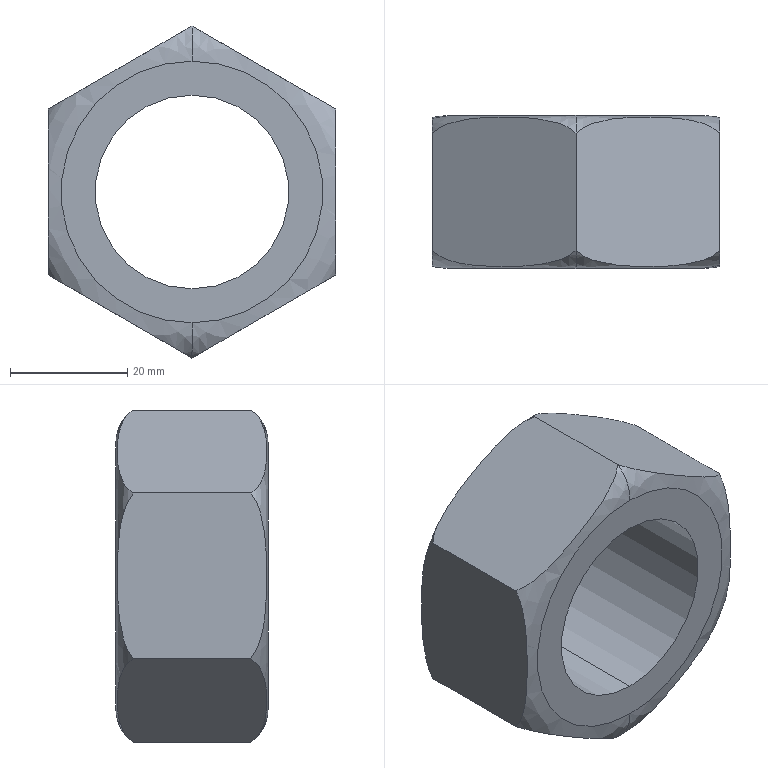Part | SolidWorks | features Extrusion 1, RevCut 1 | 1 solid | 14 faces | box 49 x 26 x 56.58 mm | volume 31477 mm3 | plane 8 | spline 4 | cylinder 2 | commonest cylinder face diameters 33 x2
STEP:
#1=CARTESIAN_POINT('',(0.,10.,-28.29));
#2=VERTEX_POINT('',#1);
#3=CARTESIAN_POINT('',(24.5,10.,-14.145));
#4=VERTEX_POINT('',#3);
#5=CARTESIAN_POINT('',(0.,10.,-28.29));
#6=CARTESIAN_POINT('',(0.412,10.401,-28.052));
#7=CARTESIAN_POINT('',(0.863,10.721,-27.792));
#8=CARTESIAN_POINT('',(1.576,11.123,-27.38));
#9=CARTESIAN_POINT('',(1.819,11.244,-27.24));
#10=CARTESIAN_POINT('',(2.317,11.465,-26.952));
#11=CARTESIAN_POINT('',(2.571,11.564,-26.806));
#12=CARTESIAN_POINT('',(3.333,11.832,-26.366));
#13=CARTESIAN_POINT('',(3.846,11.972,-26.069));
#14=CARTESIAN_POINT('',(4.88,12.204,-25.473));
#15=CARTESIAN_POINT('',(5.4,12.295,-25.173));
#16=CARTESIAN_POINT('',(6.967,12.519,-24.268));
#17=CARTESIAN_POINT('',(8.022,12.604,-23.659));
#18=CARTESIAN_POINT('',(10.136,12.711,-22.438));
#19=CARTESIAN_POINT('',(11.193,12.733,-21.828));
#20=CARTESIAN_POINT('',(13.306,12.733,-20.608));
#21=CARTESIAN_POINT('',(14.363,12.711,-19.998));
#22=CARTESIAN_POINT('',(16.475,12.604,-18.778));
#23=CARTESIAN_POINT('',(17.532,12.519,-18.168));
#24=CARTESIAN_POINT('',(19.105,12.294,-17.26));
#25=CARTESIAN_POINT('',(19.627,12.202,-16.958));
#26=CARTESIAN_POINT('',(20.667,11.969,-16.358));
#27=CARTESIAN_POINT('',(21.183,11.827,-16.06));
#28=CARTESIAN_POINT('',(22.191,11.472,-15.478));
#29=CARTESIAN_POINT('',(22.684,11.259,-15.193));
#30=CARTESIAN_POINT('',(23.399,10.855,-14.781));
#31=CARTESIAN_POINT('',(23.633,10.706,-14.646));
#32=CARTESIAN_POINT('',(24.081,10.378,-14.387));
#33=CARTESIAN_POINT('',(24.296,10.199,-14.263));
#34=CARTESIAN_POINT('',(24.5,10.,-14.145));
#35=B_SPLINE_CURVE_WITH_KNOTS('',3,(#5,#6,#7,#8,#9,#10,#11,#12,#13,#14,#15,#16,#17,#18,#19,#20,#21,#22,#23,#24,#25,#26,#27,#28,#29,#30,#31,#32,#33,#34),.UNSPECIFIED.,.F.,.F.,(4,2,2,2,2,2,2,2,2,2,2,2,2,2,4),(0.,0.00183,0.002745,0.003661,0.005491,0.007321,0.01098,0.01464,0.0183,0.02196,0.02379,0.02562,0.02745,0.02837,0.02929),.UNSPECIFIED.);
#36=EDGE_CURVE('',#2,#4,#35,.T.);
#37=ORIENTED_EDGE('',*,*,#36,.F.);
#38=CARTESIAN_POINT('',(0.,13.,-22.29));
#39=VERTEX_POINT('',#38);
#40=CARTESIAN_POINT('',(0.,10.,-28.29));
#41=CARTESIAN_POINT('',(0.,12.129,-27.029));
#42=CARTESIAN_POINT('',(0.,13.,-24.712));
#43=CARTESIAN_POINT('',(0.,13.,-22.29));
#44=B_SPLINE_CURVE_WITH_KNOTS('',3,(#40,#41,#42,#43),.UNSPECIFIED.,.F.,.F.,(4,4),(0.,1.),.UNSPECIFIED.);
#45=EDGE_CURVE('',#2,#39,#44,.T.);
#46=ORIENTED_EDGE('',*,*,#45,.T.);
#47=CARTESIAN_POINT('',(0.,13.,22.29));
#48=VERTEX_POINT('',#47);
#49=CARTESIAN_POINT('',(0.,13.,0.));
#50=DIRECTION('',(0.,1.,0.));
#51=DIRECTION('',(0.,0.,1.));
#52=AXIS2_PLACEMENT_3D('',#49,#50,#51);
#53=CIRCLE('',#52,22.29);
#54=EDGE_CURVE('',#48,#39,#53,.T.);
#55=ORIENTED_EDGE('',*,*,#54,.F.);
#56=CARTESIAN_POINT('',(0.,10.,28.29));
#57=VERTEX_POINT('',#56);
#58=CARTESIAN_POINT('',(0.,10.,28.29));
#59=CARTESIAN_POINT('',(0.,12.129,27.029));
#60=CARTESIAN_POINT('',(0.,13.,24.712));
#61=CARTESIAN_POINT('',(0.,13.,22.29));
#62=B_SPLINE_CURVE_WITH_KNOTS('',3,(#58,#59,#60,#61),.UNSPECIFIED.,.F.,.F.,(4,4),(0.,1.),.UNSPECIFIED.);
#63=EDGE_CURVE('',#57,#48,#62,.T.);
#64=ORIENTED_EDGE('',*,*,#63,.F.);
#65=CARTESIAN_POINT('',(24.5,10.,14.145));
#66=VERTEX_POINT('',#65);
#67=CARTESIAN_POINT('',(24.5,10.,14.145));
#68=CARTESIAN_POINT('',(24.088,10.401,14.383));
#69=CARTESIAN_POINT('',(23.637,10.721,14.643));
#70=CARTESIAN_POINT('',(22.924,11.123,15.055));
#71=CARTESIAN_POINT('',(22.681,11.244,15.196));
#72=CARTESIAN_POINT('',(22.183,11.465,15.483));
#73=CARTESIAN_POINT('',(21.929,11.564,15.629));
#74=CARTESIAN_POINT('',(21.167,11.832,16.069));
#75=CARTESIAN_POINT('',(20.654,11.972,16.366));
#76=CARTESIAN_POINT('',(19.62,12.204,16.962));
#77=CARTESIAN_POINT('',(19.1,12.295,17.263));
#78=CARTESIAN_POINT('',(17.533,12.519,18.168));
#79=CARTESIAN_POINT('',(16.478,12.604,18.777));
#80=CARTESIAN_POINT('',(14.364,12.711,19.997));
#81=CARTESIAN_POINT('',(13.307,12.733,20.607));
#82=CARTESIAN_POINT('',(11.194,12.733,21.827));
#83=CARTESIAN_POINT('',(10.137,12.711,22.437));
#84=CARTESIAN_POINT('',(8.025,12.604,23.657));
#85=CARTESIAN_POINT('',(6.968,12.519,24.267));
#86=CARTESIAN_POINT('',(5.395,12.294,25.175));
#87=CARTESIAN_POINT('',(4.873,12.202,25.477));
#88=CARTESIAN_POINT('',(3.833,11.969,26.077));
#89=CARTESIAN_POINT('',(3.317,11.827,26.375));
#90=CARTESIAN_POINT('',(2.309,11.472,26.957));
#91=CARTESIAN_POINT('',(1.816,11.259,27.242));
#92=CARTESIAN_POINT('',(1.101,10.855,27.654));
#93=CARTESIAN_POINT('',(0.867,10.706,27.79));
#94=CARTESIAN_POINT('',(0.419,10.378,28.048));
#95=CARTESIAN_POINT('',(0.2039,10.199,28.172));
#96=CARTESIAN_POINT('',(0.,10.,28.29));
#97=B_SPLINE_CURVE_WITH_KNOTS('',3,(#67,#68,#69,#70,#71,#72,#73,#74,#75,#76,#77,#78,#79,#80,#81,#82,#83,#84,#85,#86,#87,#88,#89,#90,#91,#92,#93,#94,#95,#96),.UNSPECIFIED.,.F.,.F.,(4,2,2,2,2,2,2,2,2,2,2,2,2,2,4),(0.,0.00183,0.002745,0.003661,0.005491,0.007321,0.01098,0.01464,0.0183,0.02196,0.02379,0.02562,0.02745,0.02837,0.02929),.UNSPECIFIED.);
#98=EDGE_CURVE('',#66,#57,#97,.T.);
#99=ORIENTED_EDGE('',*,*,#98,.F.);
#100=CARTESIAN_POINT('',(24.5,10.,-14.145));
#101=CARTESIAN_POINT('',(24.5,10.401,-13.669));
#102=CARTESIAN_POINT('',(24.5,10.721,-13.149));
#103=CARTESIAN_POINT('',(24.5,11.123,-12.326));
#104=CARTESIAN_POINT('',(24.5,11.244,-12.044));
#105=CARTESIAN_POINT('',(24.5,11.465,-11.469));
#106=CARTESIAN_POINT('',(24.5,11.564,-11.176));
#107=CARTESIAN_POINT('',(24.5,11.832,-10.296));
#108=CARTESIAN_POINT('',(24.5,11.972,-9.704));
#109=CARTESIAN_POINT('',(24.5,12.204,-8.51));
#110=CARTESIAN_POINT('',(24.5,12.295,-7.91));
#111=CARTESIAN_POINT('',(24.5,12.519,-6.1));
#112=CARTESIAN_POINT('',(24.5,12.604,-4.882));
#113=CARTESIAN_POINT('',(24.5,12.711,-2.441));
#114=CARTESIAN_POINT('',(24.5,12.733,-1.221));
#115=CARTESIAN_POINT('',(24.5,12.733,1.219));
#116=CARTESIAN_POINT('',(24.5,12.711,2.439));
#117=CARTESIAN_POINT('',(24.5,12.604,4.879));
#118=CARTESIAN_POINT('',(24.5,12.519,6.1));
#119=CARTESIAN_POINT('',(24.5,12.294,7.916));
#120=CARTESIAN_POINT('',(24.5,12.202,8.519));
#121=CARTESIAN_POINT('',(24.5,11.969,9.719));
#122=CARTESIAN_POINT('',(24.5,11.827,10.315));
#123=CARTESIAN_POINT('',(24.5,11.472,11.479));
#124=CARTESIAN_POINT('',(24.5,11.259,12.048));
#125=CARTESIAN_POINT('',(24.5,10.855,12.874));
#126=CARTESIAN_POINT('',(24.5,10.706,13.144));
#127=CARTESIAN_POINT('',(24.5,10.378,13.661));
#128=CARTESIAN_POINT('',(24.5,10.199,13.91));
#129=CARTESIAN_POINT('',(24.5,10.,14.145));
#130=B_SPLINE_CURVE_WITH_KNOTS('',3,(#100,#101,#102,#103,#104,#105,#106,#107,#108,#109,#110,#111,#112,#113,#114,#115,#116,#117,#118,#119,#120,#121,#122,#123,#124,#125,#126,#127,#128,#129),.UNSPECIFIED.,.F.,.F.,(4,2,2,2,2,2,2,2,2,2,2,2,2,2,4),(0.,0.00183,0.002745,0.003661,0.005491,0.007321,0.01098,0.01464,0.0183,0.02196,0.02379,0.02562,0.02745,0.02837,0.02929),.UNSPECIFIED.);
#131=EDGE_CURVE('',#4,#66,#130,.T.);
#132=ORIENTED_EDGE('',*,*,#131,.F.);
#133=EDGE_LOOP('',(#37,#46,#55,#64,#99,#132));
#134=FACE_OUTER_BOUND('',#133,.T.);
#135=CARTESIAN_POINT('',(0.,10.,28.29));
#136=CARTESIAN_POINT('',(56.58,10.,28.29));
#137=CARTESIAN_POINT('',(56.58,10.,-28.29));
#138=CARTESIAN_POINT('',(0.,10.,-28.29));
#139=CARTESIAN_POINT('',(0.,12.129,27.029));
#140=CARTESIAN_POINT('',(54.057,12.129,27.029));
#141=CARTESIAN_POINT('',(54.057,12.129,-27.029));
#142=CARTESIAN_POINT('',(0.,12.129,-27.029));
#143=CARTESIAN_POINT('',(0.,13.,24.712));
#144=CARTESIAN_POINT('',(49.423,13.,24.712));
#145=CARTESIAN_POINT('',(49.423,13.,-24.712));
#146=CARTESIAN_POINT('',(0.,13.,-24.712));
#147=CARTESIAN_POINT('',(0.,13.,22.29));
#148=CARTESIAN_POINT('',(44.58,13.,22.29));
#149=CARTESIAN_POINT('',(44.58,13.,-22.29));
#150=CARTESIAN_POINT('',(0.,13.,-22.29));
#151=(BOUNDED_SURFACE()B_SPLINE_SURFACE(3,3,((#135,#136,#137,#138),(#139,#140,#141,#142),(#143,#144,#145,#146),(#147,#148,#149,#150)),.UNSPECIFIED.,.F.,.F.,.F.)B_SPLINE_SURFACE_WITH_KNOTS((4,4),(4,4),(0.,1.),(0.,1.),.UNSPECIFIED.)GEOMETRIC_REPRESENTATION_ITEM()RATIONAL_B_SPLINE_SURFACE(((1.,0.3333,0.3333,1.),(1.,0.3333,0.3333,1.),(1.,0.3333,0.3333,1.),(1.,0.3333,0.3333,1.)))REPRESENTATION_ITEM('')SURFACE());
#152=ADVANCED_FACE('',(#134),#151,.F.);
#153=CARTESIAN_POINT('',(0.,-13.,22.29));
#154=VERTEX_POINT('',#153);
#155=CARTESIAN_POINT('',(0.,-13.,-22.29));
#156=VERTEX_POINT('',#155);
#157=CARTESIAN_POINT('',(0.,-13.,0.));
#158=DIRECTION('',(0.,1.,0.));
#159=DIRECTION('',(0.,0.,1.));
#160=AXIS2_PLACEMENT_3D('',#157,#158,#159);
#161=CIRCLE('',#160,22.29);
#162=EDGE_CURVE('',#154,#156,#161,.T.);
#163=ORIENTED_EDGE('',*,*,#162,.T.);
#164=CARTESIAN_POINT('',(0.,-10.,-28.29));
#165=VERTEX_POINT('',#164);
#166=CARTESIAN_POINT('',(0.,-13.,-22.29));
#167=CARTESIAN_POINT('',(0.,-13.,-24.712));
#168=CARTESIAN_POINT('',(0.,-12.129,-27.029));
#169=CARTESIAN_POINT('',(0.,-10.,-28.29));
#170=B_SPLINE_CURVE_WITH_KNOTS('',3,(#166,#167,#168,#169),.UNSPECIFIED.,.F.,.F.,(4,4),(0.,1.),.UNSPECIFIED.);
#171=EDGE_CURVE('',#156,#165,#170,.T.);
#172=ORIENTED_EDGE('',*,*,#171,.T.);
#173=CARTESIAN_POINT('',(24.5,-10.,-14.145));
#174=VERTEX_POINT('',#173);
#175=CARTESIAN_POINT('',(24.5,-10.,-14.145));
#176=CARTESIAN_POINT('',(24.088,-10.401,-14.383));
#177=CARTESIAN_POINT('',(23.637,-10.721,-14.643));
#178=CARTESIAN_POINT('',(22.924,-11.123,-15.055));
#179=CARTESIAN_POINT('',(22.681,-11.244,-15.196));
#180=CARTESIAN_POINT('',(22.183,-11.465,-15.483));
#181=CARTESIAN_POINT('',(21.929,-11.564,-15.629));
#182=CARTESIAN_POINT('',(21.167,-11.832,-16.069));
#183=CARTESIAN_POINT('',(20.654,-11.972,-16.366));
#184=CARTESIAN_POINT('',(19.62,-12.204,-16.962));
#185=CARTESIAN_POINT('',(19.1,-12.295,-17.263));
#186=CARTESIAN_POINT('',(17.533,-12.519,-18.168));
#187=CARTESIAN_POINT('',(16.478,-12.604,-18.777));
#188=CARTESIAN_POINT('',(14.364,-12.711,-19.997));
#189=CARTESIAN_POINT('',(13.307,-12.733,-20.607));
#190=CARTESIAN_POINT('',(11.194,-12.733,-21.827));
#191=CARTESIAN_POINT('',(10.137,-12.711,-22.437));
#192=CARTESIAN_POINT('',(8.025,-12.604,-23.657));
#193=CARTESIAN_POINT('',(6.968,-12.519,-24.267));
#194=CARTESIAN_POINT('',(5.395,-12.294,-25.175));
#195=CARTESIAN_POINT('',(4.873,-12.202,-25.477));
#196=CARTESIAN_POINT('',(3.833,-11.969,-26.077));
#197=CARTESIAN_POINT('',(3.317,-11.827,-26.375));
#198=CARTESIAN_POINT('',(2.309,-11.472,-26.957));
#199=CARTESIAN_POINT('',(1.816,-11.259,-27.242));
#200=CARTESIAN_POINT('',(1.101,-10.855,-27.654));
#201=CARTESIAN_POINT('',(0.867,-10.706,-27.79));
#202=CARTESIAN_POINT('',(0.419,-10.378,-28.048));
#203=CARTESIAN_POINT('',(0.2039,-10.199,-28.172));
#204=CARTESIAN_POINT('',(0.,-10.,-28.29));
#205=B_SPLINE_CURVE_WITH_KNOTS('',3,(#175,#176,#177,#178,#179,#180,#181,#182,#183,#184,#185,#186,#187,#188,#189,#190,#191,#192,#193,#194,#195,#196,#197,#198,#199,#200,#201,#202,#203,#204),.UNSPECIFIED.,.F.,.F.,(4,2,2,2,2,2,2,2,2,2,2,2,2,2,4),(0.,0.00183,0.002745,0.003661,0.005491,0.007321,0.01098,0.01464,0.0183,0.02196,0.02379,0.02562,0.02745,0.02837,0.02929),.UNSPECIFIED.);
#206=EDGE_CURVE('',#174,#165,#205,.T.);
#207=ORIENTED_EDGE('',*,*,#206,.F.);
#208=CARTESIAN_POINT('',(24.5,-10.,14.145));
#209=VERTEX_POINT('',#208);
#210=CARTESIAN_POINT('',(24.5,-10.,14.145));
#211=CARTESIAN_POINT('',(24.5,-10.401,13.669));
#212=CARTESIAN_POINT('',(24.5,-10.721,13.149));
#213=CARTESIAN_POINT('',(24.5,-11.123,12.326));
#214=CARTESIAN_POINT('',(24.5,-11.244,12.044));
#215=CARTESIAN_POINT('',(24.5,-11.465,11.469));
#216=CARTESIAN_POINT('',(24.5,-11.564,11.176));
#217=CARTESIAN_POINT('',(24.5,-11.832,10.296));
#218=CARTESIAN_POINT('',(24.5,-11.972,9.704));
#219=CARTESIAN_POINT('',(24.5,-12.204,8.51));
#220=CARTESIAN_POINT('',(24.5,-12.295,7.91));
#221=CARTESIAN_POINT('',(24.5,-12.519,6.1));
#222=CARTESIAN_POINT('',(24.5,-12.604,4.882));
#223=CARTESIAN_POINT('',(24.5,-12.711,2.441));
#224=CARTESIAN_POINT('',(24.5,-12.733,1.221));
#225=CARTESIAN_POINT('',(24.5,-12.733,-1.219));
#226=CARTESIAN_POINT('',(24.5,-12.711,-2.439));
#227=CARTESIAN_POINT('',(24.5,-12.604,-4.879));
#228=CARTESIAN_POINT('',(24.5,-12.519,-6.1));
#229=CARTESIAN_POINT('',(24.5,-12.294,-7.916));
#230=CARTESIAN_POINT('',(24.5,-12.202,-8.519));
#231=CARTESIAN_POINT('',(24.5,-11.969,-9.719));
#232=CARTESIAN_POINT('',(24.5,-11.827,-10.315));
#233=CARTESIAN_POINT('',(24.5,-11.472,-11.479));
#234=CARTESIAN_POINT('',(24.5,-11.259,-12.048));
#235=CARTESIAN_POINT('',(24.5,-10.855,-12.874));
#236=CARTESIAN_POINT('',(24.5,-10.706,-13.144));
#237=CARTESIAN_POINT('',(24.5,-10.378,-13.661));
#238=CARTESIAN_POINT('',(24.5,-10.199,-13.91));
#239=CARTESIAN_POINT('',(24.5,-10.,-14.145));
#240=B_SPLINE_CURVE_WITH_KNOTS('',3,(#210,#211,#212,#213,#214,#215,#216,#217,#218,#219,#220,#221,#222,#223,#224,#225,#226,#227,#228,#229,#230,#231,#232,#233,#234,#235,#236,#237,#238,#239),.UNSPECIFIED.,.F.,.F.,(4,2,2,2,2,2,2,2,2,2,2,2,2,2,4),(0.,0.00183,0.002745,0.003661,0.005491,0.007321,0.01098,0.01464,0.0183,0.02196,0.02379,0.02562,0.02745,0.02837,0.02929),.UNSPECIFIED.);
#241=EDGE_CURVE('',#209,#174,#240,.T.);
#242=ORIENTED_EDGE('',*,*,#241,.F.);
#243=CARTESIAN_POINT('',(0.,-10.,28.29));
#244=VERTEX_POINT('',#243);
#245=CARTESIAN_POINT('',(0.,-10.,28.29));
#246=CARTESIAN_POINT('',(0.412,-10.401,28.052));
#247=CARTESIAN_POINT('',(0.863,-10.721,27.792));
#248=CARTESIAN_POINT('',(1.576,-11.123,27.38));
#249=CARTESIAN_POINT('',(1.819,-11.244,27.24));
#250=CARTESIAN_POINT('',(2.317,-11.465,26.952));
#251=CARTESIAN_POINT('',(2.571,-11.564,26.806));
#252=CARTESIAN_POINT('',(3.333,-11.832,26.366));
#253=CARTESIAN_POINT('',(3.846,-11.972,26.069));
#254=CARTESIAN_POINT('',(4.88,-12.204,25.473));
#255=CARTESIAN_POINT('',(5.4,-12.295,25.173));
#256=CARTESIAN_POINT('',(6.967,-12.519,24.268));
#257=CARTESIAN_POINT('',(8.022,-12.604,23.659));
#258=CARTESIAN_POINT('',(10.136,-12.711,22.438));
#259=CARTESIAN_POINT('',(11.193,-12.733,21.828));
#260=CARTESIAN_POINT('',(13.306,-12.733,20.608));
#261=CARTESIAN_POINT('',(14.363,-12.711,19.998));
#262=CARTESIAN_POINT('',(16.475,-12.604,18.778));
#263=CARTESIAN_POINT('',(17.532,-12.519,18.168));
#264=CARTESIAN_POINT('',(19.105,-12.294,17.26));
#265=CARTESIAN_POINT('',(19.627,-12.202,16.958));
#266=CARTESIAN_POINT('',(20.667,-11.969,16.358));
#267=CARTESIAN_POINT('',(21.183,-11.827,16.06));
#268=CARTESIAN_POINT('',(22.191,-11.472,15.478));
#269=CARTESIAN_POINT('',(22.684,-11.259,15.193));
#270=CARTESIAN_POINT('',(23.399,-10.855,14.781));
#271=CARTESIAN_POINT('',(23.633,-10.706,14.646));
#272=CARTESIAN_POINT('',(24.081,-10.378,14.387));
#273=CARTESIAN_POINT('',(24.296,-10.199,14.263));
#274=CARTESIAN_POINT('',(24.5,-10.,14.145));
#275=B_SPLINE_CURVE_WITH_KNOTS('',3,(#245,#246,#247,#248,#249,#250,#251,#252,#253,#254,#255,#256,#257,#258,#259,#260,#261,#262,#263,#264,#265,#266,#267,#268,#269,#270,#271,#272,#273,#274),.UNSPECIFIED.,.F.,.F.,(4,2,2,2,2,2,2,2,2,2,2,2,2,2,4),(0.,0.00183,0.002745,0.003661,0.005491,0.007321,0.01098,0.01464,0.0183,0.02196,0.02379,0.02562,0.02745,0.02837,0.02929),.UNSPECIFIED.);
#276=EDGE_CURVE('',#244,#209,#275,.T.);
#277=ORIENTED_EDGE('',*,*,#276,.F.);
#278=CARTESIAN_POINT('',(0.,-13.,22.29));
#279=CARTESIAN_POINT('',(0.,-13.,24.712));
#280=CARTESIAN_POINT('',(0.,-12.129,27.029));
#281=CARTESIAN_POINT('',(0.,-10.,28.29));
#282=B_SPLINE_CURVE_WITH_KNOTS('',3,(#278,#279,#280,#281),.UNSPECIFIED.,.F.,.F.,(4,4),(0.,1.),.UNSPECIFIED.);
#283=EDGE_CURVE('',#154,#244,#282,.T.);
#284=ORIENTED_EDGE('',*,*,#283,.F.);
#285=EDGE_LOOP('',(#163,#172,#207,#242,#277,#284));
#286=FACE_OUTER_BOUND('',#285,.T.);
#287=CARTESIAN_POINT('',(0.,-13.,22.29));
#288=CARTESIAN_POINT('',(44.58,-13.,22.29));
#289=CARTESIAN_POINT('',(44.58,-13.,-22.29));
#290=CARTESIAN_POINT('',(0.,-13.,-22.29));
#291=CARTESIAN_POINT('',(0.,-13.,24.712));
#292=CARTESIAN_POINT('',(49.423,-13.,24.712));
#293=CARTESIAN_POINT('',(49.423,-13.,-24.712));
#294=CARTESIAN_POINT('',(0.,-13.,-24.712));
#295=CARTESIAN_POINT('',(0.,-12.129,27.029));
#296=CARTESIAN_POINT('',(54.057,-12.129,27.029));
#297=CARTESIAN_POINT('',(54.057,-12.129,-27.029));
#298=CARTESIAN_POINT('',(0.,-12.129,-27.029));
#299=CARTESIAN_POINT('',(0.,-10.,28.29));
#300=CARTESIAN_POINT('',(56.58,-10.,28.29));
#301=CARTESIAN_POINT('',(56.58,-10.,-28.29));
#302=CARTESIAN_POINT('',(0.,-10.,-28.29));
#303=(BOUNDED_SURFACE()B_SPLINE_SURFACE(3,3,((#287,#288,#289,#290),(#291,#292,#293,#294),(#295,#296,#297,#298),(#299,#300,#301,#302)),.UNSPECIFIED.,.F.,.F.,.F.)B_SPLINE_SURFACE_WITH_KNOTS((4,4),(4,4),(0.,1.),(0.,1.),.UNSPECIFIED.)GEOMETRIC_REPRESENTATION_ITEM()RATIONAL_B_SPLINE_SURFACE(((1.,0.3333,0.3333,1.),(1.,0.3333,0.3333,1.),(1.,0.3333,0.3333,1.),(1.,0.3333,0.3333,1.)))REPRESENTATION_ITEM('')SURFACE());
#304=ADVANCED_FACE('',(#286),#303,.F.);
#305=CARTESIAN_POINT('',(0.,13.,-16.5));
#306=VERTEX_POINT('',#305);
#307=CARTESIAN_POINT('',(0.,13.,16.5));
#308=VERTEX_POINT('',#307);
#309=CARTESIAN_POINT('',(0.,13.,0.));
#310=DIRECTION('',(0.,1.,0.));
#311=DIRECTION('',(0.,0.,1.));
#312=AXIS2_PLACEMENT_3D('',#309,#310,#311);
#313=CIRCLE('',#312,16.5);
#314=EDGE_CURVE('',#306,#308,#313,.T.);
#315=ORIENTED_EDGE('',*,*,#314,.T.);
#316=CARTESIAN_POINT('',(0.,-13.,16.5));
#317=VERTEX_POINT('',#316);
#318=CARTESIAN_POINT('',(0.,13.,16.5));
#319=DIRECTION('',(0.,-1.,0.));
#320=VECTOR('',#319,1000.);
#321=LINE('',#318,#320);
#322=EDGE_CURVE('',#308,#317,#321,.T.);
#323=ORIENTED_EDGE('',*,*,#322,.T.);
#324=CARTESIAN_POINT('',(0.,-13.,-16.5));
#325=VERTEX_POINT('',#324);
#326=CARTESIAN_POINT('',(0.,-13.,0.));
#327=DIRECTION('',(0.,1.,0.));
#328=DIRECTION('',(0.,0.,1.));
#329=AXIS2_PLACEMENT_3D('',#326,#327,#328);
#330=CIRCLE('',#329,16.5);
#331=EDGE_CURVE('',#325,#317,#330,.T.);
#332=ORIENTED_EDGE('',*,*,#331,.F.);
#333=CARTESIAN_POINT('',(0.,13.,-16.5));
#334=DIRECTION('',(0.,-1.,0.));
#335=VECTOR('',#334,1000.);
#336=LINE('',#333,#335);
#337=EDGE_CURVE('',#306,#325,#336,.T.);
#338=ORIENTED_EDGE('',*,*,#337,.F.);
#339=EDGE_LOOP('',(#315,#323,#332,#338));
#340=FACE_OUTER_BOUND('',#339,.T.);
#341=CARTESIAN_POINT('',(0.,13.,0.));
#342=DIRECTION('',(0.,-1.,0.));
#343=DIRECTION('',(0.,0.,-1.));
#344=AXIS2_PLACEMENT_3D('',#341,#342,#343);
#345=CYLINDRICAL_SURFACE('',#344,16.5);
#346=ADVANCED_FACE('',(#340),#345,.F.);
#347=ORIENTED_EDGE('',*,*,#314,.F.);
#348=CARTESIAN_POINT('',(0.,13.,0.));
#349=DIRECTION('',(0.,1.,0.));
#350=DIRECTION('',(0.,0.,1.));
#351=AXIS2_PLACEMENT_3D('',#348,#349,#350);
#352=CIRCLE('',#351,16.5);
#353=EDGE_CURVE('',#308,#306,#352,.T.);
#354=ORIENTED_EDGE('',*,*,#353,.F.);
#355=EDGE_LOOP('',(#347,#354));
#356=FACE_BOUND('',#355,.T.);
#357=ORIENTED_EDGE('',*,*,#54,.T.);
#358=CARTESIAN_POINT('',(0.,13.,0.));
#359=DIRECTION('',(0.,1.,0.));
#360=DIRECTION('',(0.,0.,1.));
#361=AXIS2_PLACEMENT_3D('',#358,#359,#360);
#362=CIRCLE('',#361,22.29);
#363=EDGE_CURVE('',#39,#48,#362,.T.);
#364=ORIENTED_EDGE('',*,*,#363,.T.);
#365=EDGE_LOOP('',(#357,#364));
#366=FACE_OUTER_BOUND('',#365,.T.);
#367=CARTESIAN_POINT('',(0.,13.,0.));
#368=DIRECTION('',(0.,1.,0.));
#369=DIRECTION('',(0.,0.,1.));
#370=AXIS2_PLACEMENT_3D('',#367,#368,#369);
#371=PLANE('',#370);
#372=ADVANCED_FACE('',(#356,#366),#371,.T.);
#373=ORIENTED_EDGE('',*,*,#331,.T.);
#374=CARTESIAN_POINT('',(0.,-13.,0.));
#375=DIRECTION('',(0.,1.,0.));
#376=DIRECTION('',(0.,0.,1.));
#377=AXIS2_PLACEMENT_3D('',#374,#375,#376);
#378=CIRCLE('',#377,16.5);
#379=EDGE_CURVE('',#317,#325,#378,.T.);
#380=ORIENTED_EDGE('',*,*,#379,.T.);
#381=EDGE_LOOP('',(#373,#380));
#382=FACE_BOUND('',#381,.T.);
#383=ORIENTED_EDGE('',*,*,#162,.F.);
#384=CARTESIAN_POINT('',(0.,-13.,0.));
#385=DIRECTION('',(0.,1.,0.));
#386=DIRECTION('',(0.,0.,1.));
#387=AXIS2_PLACEMENT_3D('',#384,#385,#386);
#388=CIRCLE('',#387,22.29);
#389=EDGE_CURVE('',#156,#154,#388,.T.);
#390=ORIENTED_EDGE('',*,*,#389,.F.);
#391=EDGE_LOOP('',(#383,#390));
#392=FACE_OUTER_BOUND('',#391,.T.);
#393=CARTESIAN_POINT('',(0.,-13.,0.));
#394=DIRECTION('',(0.,1.,0.));
#395=DIRECTION('',(0.,0.,1.));
#396=AXIS2_PLACEMENT_3D('',#393,#394,#395);
#397=PLANE('',#396);
#398=ADVANCED_FACE('',(#382,#392),#397,.F.);
#399=ORIENTED_EDGE('',*,*,#322,.F.);
#400=ORIENTED_EDGE('',*,*,#353,.T.);
#401=ORIENTED_EDGE('',*,*,#337,.T.);
#402=ORIENTED_EDGE('',*,*,#379,.F.);
#403=EDGE_LOOP('',(#399,#400,#401,#402));
#404=FACE_OUTER_BOUND('',#403,.T.);
#405=CARTESIAN_POINT('',(0.,13.,0.));
#406=DIRECTION('',(0.,-1.,0.));
#407=DIRECTION('',(0.,0.,-1.));
#408=AXIS2_PLACEMENT_3D('',#405,#406,#407);
#409=CYLINDRICAL_SURFACE('',#408,16.5);
#410=ADVANCED_FACE('',(#404),#409,.F.);
#411=ORIENTED_EDGE('',*,*,#171,.F.);
#412=ORIENTED_EDGE('',*,*,#389,.T.);
#413=ORIENTED_EDGE('',*,*,#283,.T.);
#414=CARTESIAN_POINT('',(-24.5,-10.,14.145));
#415=VERTEX_POINT('',#414);
#416=CARTESIAN_POINT('',(-24.5,-10.,14.145));
#417=CARTESIAN_POINT('',(-24.088,-10.401,14.383));
#418=CARTESIAN_POINT('',(-23.637,-10.721,14.643));
#419=CARTESIAN_POINT('',(-22.924,-11.123,15.055));
#420=CARTESIAN_POINT('',(-22.681,-11.244,15.196));
#421=CARTESIAN_POINT('',(-22.183,-11.465,15.483));
#422=CARTESIAN_POINT('',(-21.929,-11.564,15.629));
#423=CARTESIAN_POINT('',(-21.167,-11.832,16.069));
#424=CARTESIAN_POINT('',(-20.654,-11.972,16.366));
#425=CARTESIAN_POINT('',(-19.62,-12.204,16.962));
#426=CARTESIAN_POINT('',(-19.1,-12.295,17.263));
#427=CARTESIAN_POINT('',(-17.533,-12.519,18.168));
#428=CARTESIAN_POINT('',(-16.478,-12.604,18.777));
#429=CARTESIAN_POINT('',(-14.364,-12.711,19.997));
#430=CARTESIAN_POINT('',(-13.307,-12.733,20.607));
#431=CARTESIAN_POINT('',(-11.194,-12.733,21.827));
#432=CARTESIAN_POINT('',(-10.137,-12.711,22.437));
#433=CARTESIAN_POINT('',(-8.025,-12.604,23.657));
#434=CARTESIAN_POINT('',(-6.968,-12.519,24.267));
#435=CARTESIAN_POINT('',(-5.395,-12.294,25.175));
#436=CARTESIAN_POINT('',(-4.873,-12.202,25.477));
#437=CARTESIAN_POINT('',(-3.833,-11.969,26.077));
#438=CARTESIAN_POINT('',(-3.317,-11.827,26.375));
#439=CARTESIAN_POINT('',(-2.309,-11.472,26.957));
#440=CARTESIAN_POINT('',(-1.816,-11.259,27.242));
#441=CARTESIAN_POINT('',(-1.101,-10.855,27.654));
#442=CARTESIAN_POINT('',(-0.867,-10.706,27.79));
#443=CARTESIAN_POINT('',(-0.419,-10.378,28.048));
#444=CARTESIAN_POINT('',(-0.2039,-10.199,28.172));
#445=CARTESIAN_POINT('',(0.,-10.,28.29));
#446=B_SPLINE_CURVE_WITH_KNOTS('',3,(#416,#417,#418,#419,#420,#421,#422,#423,#424,#425,#426,#427,#428,#429,#430,#431,#432,#433,#434,#435,#436,#437,#438,#439,#440,#441,#442,#443,#444,#445),.UNSPECIFIED.,.F.,.F.,(4,2,2,2,2,2,2,2,2,2,2,2,2,2,4),(0.,0.00183,0.002745,0.003661,0.005491,0.007321,0.01098,0.01464,0.0183,0.02196,0.02379,0.02562,0.02745,0.02837,0.02929),.UNSPECIFIED.);
#447=EDGE_CURVE('',#415,#244,#446,.T.);
#448=ORIENTED_EDGE('',*,*,#447,.F.);
#449=CARTESIAN_POINT('',(-24.5,-10.,-14.145));
#450=VERTEX_POINT('',#449);
#451=CARTESIAN_POINT('',(-24.5,-10.,-14.145));
#452=CARTESIAN_POINT('',(-24.5,-10.401,-13.669));
#453=CARTESIAN_POINT('',(-24.5,-10.721,-13.149));
#454=CARTESIAN_POINT('',(-24.5,-11.123,-12.326));
#455=CARTESIAN_POINT('',(-24.5,-11.244,-12.044));
#456=CARTESIAN_POINT('',(-24.5,-11.465,-11.469));
#457=CARTESIAN_POINT('',(-24.5,-11.564,-11.176));
#458=CARTESIAN_POINT('',(-24.5,-11.832,-10.296));
#459=CARTESIAN_POINT('',(-24.5,-11.972,-9.704));
#460=CARTESIAN_POINT('',(-24.5,-12.204,-8.51));
#461=CARTESIAN_POINT('',(-24.5,-12.295,-7.91));
#462=CARTESIAN_POINT('',(-24.5,-12.519,-6.1));
#463=CARTESIAN_POINT('',(-24.5,-12.604,-4.882));
#464=CARTESIAN_POINT('',(-24.5,-12.711,-2.441));
#465=CARTESIAN_POINT('',(-24.5,-12.733,-1.221));
#466=CARTESIAN_POINT('',(-24.5,-12.733,1.219));
#467=CARTESIAN_POINT('',(-24.5,-12.711,2.439));
#468=CARTESIAN_POINT('',(-24.5,-12.604,4.879));
#469=CARTESIAN_POINT('',(-24.5,-12.519,6.1));
#470=CARTESIAN_POINT('',(-24.5,-12.294,7.916));
#471=CARTESIAN_POINT('',(-24.5,-12.202,8.519));
#472=CARTESIAN_POINT('',(-24.5,-11.969,9.719));
#473=CARTESIAN_POINT('',(-24.5,-11.827,10.315));
#474=CARTESIAN_POINT('',(-24.5,-11.472,11.479));
#475=CARTESIAN_POINT('',(-24.5,-11.259,12.048));
#476=CARTESIAN_POINT('',(-24.5,-10.855,12.874));
#477=CARTESIAN_POINT('',(-24.5,-10.706,13.144));
#478=CARTESIAN_POINT('',(-24.5,-10.378,13.661));
#479=CARTESIAN_POINT('',(-24.5,-10.199,13.91));
#480=CARTESIAN_POINT('',(-24.5,-10.,14.145));
#481=B_SPLINE_CURVE_WITH_KNOTS('',3,(#451,#452,#453,#454,#455,#456,#457,#458,#459,#460,#461,#462,#463,#464,#465,#466,#467,#468,#469,#470,#471,#472,#473,#474,#475,#476,#477,#478,#479,#480),.UNSPECIFIED.,.F.,.F.,(4,2,2,2,2,2,2,2,2,2,2,2,2,2,4),(0.,0.00183,0.002745,0.003661,0.005491,0.007321,0.01098,0.01464,0.0183,0.02196,0.02379,0.02562,0.02745,0.02837,0.02929),.UNSPECIFIED.);
#482=EDGE_CURVE('',#450,#415,#481,.T.);
#483=ORIENTED_EDGE('',*,*,#482,.F.);
#484=CARTESIAN_POINT('',(0.,-10.,-28.29));
#485=CARTESIAN_POINT('',(-0.412,-10.401,-28.052));
#486=CARTESIAN_POINT('',(-0.863,-10.721,-27.792));
#487=CARTESIAN_POINT('',(-1.576,-11.123,-27.38));
#488=CARTESIAN_POINT('',(-1.819,-11.244,-27.24));
#489=CARTESIAN_POINT('',(-2.317,-11.465,-26.952));
#490=CARTESIAN_POINT('',(-2.571,-11.564,-26.806));
#491=CARTESIAN_POINT('',(-3.333,-11.832,-26.366));
#492=CARTESIAN_POINT('',(-3.846,-11.972,-26.069));
#493=CARTESIAN_POINT('',(-4.88,-12.204,-25.473));
#494=CARTESIAN_POINT('',(-5.4,-12.295,-25.173));
#495=CARTESIAN_POINT('',(-6.967,-12.519,-24.268));
#496=CARTESIAN_POINT('',(-8.022,-12.604,-23.659));
#497=CARTESIAN_POINT('',(-10.136,-12.711,-22.438));
#498=CARTESIAN_POINT('',(-11.193,-12.733,-21.828));
#499=CARTESIAN_POINT('',(-13.306,-12.733,-20.608));
#500=CARTESIAN_POINT('',(-14.363,-12.711,-19.998));
#501=CARTESIAN_POINT('',(-16.475,-12.604,-18.778));
#502=CARTESIAN_POINT('',(-17.532,-12.519,-18.168));
#503=CARTESIAN_POINT('',(-19.105,-12.294,-17.26));
#504=CARTESIAN_POINT('',(-19.627,-12.202,-16.958));
#505=CARTESIAN_POINT('',(-20.667,-11.969,-16.358));
#506=CARTESIAN_POINT('',(-21.183,-11.827,-16.06));
#507=CARTESIAN_POINT('',(-22.191,-11.472,-15.478));
#508=CARTESIAN_POINT('',(-22.684,-11.259,-15.193));
#509=CARTESIAN_POINT('',(-23.399,-10.855,-14.781));
#510=CARTESIAN_POINT('',(-23.633,-10.706,-14.646));
#511=CARTESIAN_POINT('',(-24.081,-10.378,-14.387));
#512=CARTESIAN_POINT('',(-24.296,-10.199,-14.263));
#513=CARTESIAN_POINT('',(-24.5,-10.,-14.145));
#514=B_SPLINE_CURVE_WITH_KNOTS('',3,(#484,#485,#486,#487,#488,#489,#490,#491,#492,#493,#494,#495,#496,#497,#498,#499,#500,#501,#502,#503,#504,#505,#506,#507,#508,#509,#510,#511,#512,#513),.UNSPECIFIED.,.F.,.F.,(4,2,2,2,2,2,2,2,2,2,2,2,2,2,4),(0.,0.00183,0.002745,0.003661,0.005491,0.007321,0.01098,0.01464,0.0183,0.02196,0.02379,0.02562,0.02745,0.02837,0.02929),.UNSPECIFIED.);
#515=EDGE_CURVE('',#165,#450,#514,.T.);
#516=ORIENTED_EDGE('',*,*,#515,.F.);
#517=EDGE_LOOP('',(#411,#412,#413,#448,#483,#516));
#518=FACE_OUTER_BOUND('',#517,.T.);
#519=CARTESIAN_POINT('',(0.,-13.,-22.29));
#520=CARTESIAN_POINT('',(-44.58,-13.,-22.29));
#521=CARTESIAN_POINT('',(-44.58,-13.,22.29));
#522=CARTESIAN_POINT('',(0.,-13.,22.29));
#523=CARTESIAN_POINT('',(0.,-13.,-24.712));
#524=CARTESIAN_POINT('',(-49.423,-13.,-24.712));
#525=CARTESIAN_POINT('',(-49.423,-13.,24.712));
#526=CARTESIAN_POINT('',(0.,-13.,24.712));
#527=CARTESIAN_POINT('',(0.,-12.129,-27.029));
#528=CARTESIAN_POINT('',(-54.057,-12.129,-27.029));
#529=CARTESIAN_POINT('',(-54.057,-12.129,27.029));
#530=CARTESIAN_POINT('',(0.,-12.129,27.029));
#531=CARTESIAN_POINT('',(0.,-10.,-28.29));
#532=CARTESIAN_POINT('',(-56.58,-10.,-28.29));
#533=CARTESIAN_POINT('',(-56.58,-10.,28.29));
#534=CARTESIAN_POINT('',(0.,-10.,28.29));
#535=(BOUNDED_SURFACE()B_SPLINE_SURFACE(3,3,((#519,#520,#521,#522),(#523,#524,#525,#526),(#527,#528,#529,#530),(#531,#532,#533,#534)),.UNSPECIFIED.,.F.,.F.,.F.)B_SPLINE_SURFACE_WITH_KNOTS((4,4),(4,4),(0.,1.),(0.,1.),.UNSPECIFIED.)GEOMETRIC_REPRESENTATION_ITEM()RATIONAL_B_SPLINE_SURFACE(((1.,0.3333,0.3333,1.),(1.,0.3333,0.3333,1.),(1.,0.3333,0.3333,1.),(1.,0.3333,0.3333,1.)))REPRESENTATION_ITEM('')SURFACE());
#536=ADVANCED_FACE('',(#518),#535,.F.);
#537=ORIENTED_EDGE('',*,*,#45,.F.);
#538=CARTESIAN_POINT('',(-24.5,10.,-14.145));
#539=VERTEX_POINT('',#538);
#540=CARTESIAN_POINT('',(-24.5,10.,-14.145));
#541=CARTESIAN_POINT('',(-24.088,10.401,-14.383));
#542=CARTESIAN_POINT('',(-23.637,10.721,-14.643));
#543=CARTESIAN_POINT('',(-22.924,11.123,-15.055));
#544=CARTESIAN_POINT('',(-22.681,11.244,-15.196));
#545=CARTESIAN_POINT('',(-22.183,11.465,-15.483));
#546=CARTESIAN_POINT('',(-21.929,11.564,-15.629));
#547=CARTESIAN_POINT('',(-21.167,11.832,-16.069));
#548=CARTESIAN_POINT('',(-20.654,11.972,-16.366));
#549=CARTESIAN_POINT('',(-19.62,12.204,-16.962));
#550=CARTESIAN_POINT('',(-19.1,12.295,-17.263));
#551=CARTESIAN_POINT('',(-17.533,12.519,-18.168));
#552=CARTESIAN_POINT('',(-16.478,12.604,-18.777));
#553=CARTESIAN_POINT('',(-14.364,12.711,-19.997));
#554=CARTESIAN_POINT('',(-13.307,12.733,-20.607));
#555=CARTESIAN_POINT('',(-11.194,12.733,-21.827));
#556=CARTESIAN_POINT('',(-10.137,12.711,-22.437));
#557=CARTESIAN_POINT('',(-8.025,12.604,-23.657));
#558=CARTESIAN_POINT('',(-6.968,12.519,-24.267));
#559=CARTESIAN_POINT('',(-5.395,12.294,-25.175));
#560=CARTESIAN_POINT('',(-4.873,12.202,-25.477));
#561=CARTESIAN_POINT('',(-3.833,11.969,-26.077));
#562=CARTESIAN_POINT('',(-3.317,11.827,-26.375));
#563=CARTESIAN_POINT('',(-2.309,11.472,-26.957));
#564=CARTESIAN_POINT('',(-1.816,11.259,-27.242));
#565=CARTESIAN_POINT('',(-1.101,10.855,-27.654));
#566=CARTESIAN_POINT('',(-0.867,10.706,-27.79));
#567=CARTESIAN_POINT('',(-0.419,10.378,-28.048));
#568=CARTESIAN_POINT('',(-0.2039,10.199,-28.172));
#569=CARTESIAN_POINT('',(0.,10.,-28.29));
#570=B_SPLINE_CURVE_WITH_KNOTS('',3,(#540,#541,#542,#543,#544,#545,#546,#547,#548,#549,#550,#551,#552,#553,#554,#555,#556,#557,#558,#559,#560,#561,#562,#563,#564,#565,#566,#567,#568,#569),.UNSPECIFIED.,.F.,.F.,(4,2,2,2,2,2,2,2,2,2,2,2,2,2,4),(0.,0.00183,0.002745,0.003661,0.005491,0.007321,0.01098,0.01464,0.0183,0.02196,0.02379,0.02562,0.02745,0.02837,0.02929),.UNSPECIFIED.);
#571=EDGE_CURVE('',#539,#2,#570,.T.);
#572=ORIENTED_EDGE('',*,*,#571,.F.);
#573=CARTESIAN_POINT('',(-24.5,10.,14.145));
#574=VERTEX_POINT('',#573);
#575=CARTESIAN_POINT('',(-24.5,10.,14.145));
#576=CARTESIAN_POINT('',(-24.5,10.401,13.669));
#577=CARTESIAN_POINT('',(-24.5,10.721,13.149));
#578=CARTESIAN_POINT('',(-24.5,11.123,12.326));
#579=CARTESIAN_POINT('',(-24.5,11.244,12.044));
#580=CARTESIAN_POINT('',(-24.5,11.465,11.469));
#581=CARTESIAN_POINT('',(-24.5,11.564,11.176));
#582=CARTESIAN_POINT('',(-24.5,11.832,10.296));
#583=CARTESIAN_POINT('',(-24.5,11.972,9.704));
#584=CARTESIAN_POINT('',(-24.5,12.204,8.51));
#585=CARTESIAN_POINT('',(-24.5,12.295,7.91));
#586=CARTESIAN_POINT('',(-24.5,12.519,6.1));
#587=CARTESIAN_POINT('',(-24.5,12.604,4.882));
#588=CARTESIAN_POINT('',(-24.5,12.711,2.441));
#589=CARTESIAN_POINT('',(-24.5,12.733,1.221));
#590=CARTESIAN_POINT('',(-24.5,12.733,-1.219));
#591=CARTESIAN_POINT('',(-24.5,12.711,-2.439));
#592=CARTESIAN_POINT('',(-24.5,12.604,-4.879));
#593=CARTESIAN_POINT('',(-24.5,12.519,-6.1));
#594=CARTESIAN_POINT('',(-24.5,12.294,-7.916));
#595=CARTESIAN_POINT('',(-24.5,12.202,-8.519));
#596=CARTESIAN_POINT('',(-24.5,11.969,-9.719));
#597=CARTESIAN_POINT('',(-24.5,11.827,-10.315));
#598=CARTESIAN_POINT('',(-24.5,11.472,-11.479));
#599=CARTESIAN_POINT('',(-24.5,11.259,-12.048));
#600=CARTESIAN_POINT('',(-24.5,10.855,-12.874));
#601=CARTESIAN_POINT('',(-24.5,10.706,-13.144));
#602=CARTESIAN_POINT('',(-24.5,10.378,-13.661));
#603=CARTESIAN_POINT('',(-24.5,10.199,-13.91));
#604=CARTESIAN_POINT('',(-24.5,10.,-14.145));
#605=B_SPLINE_CURVE_WITH_KNOTS('',3,(#575,#576,#577,#578,#579,#580,#581,#582,#583,#584,#585,#586,#587,#588,#589,#590,#591,#592,#593,#594,#595,#596,#597,#598,#599,#600,#601,#602,#603,#604),.UNSPECIFIED.,.F.,.F.,(4,2,2,2,2,2,2,2,2,2,2,2,2,2,4),(0.,0.00183,0.002745,0.003661,0.005491,0.007321,0.01098,0.01464,0.0183,0.02196,0.02379,0.02562,0.02745,0.02837,0.02929),.UNSPECIFIED.);
#606=EDGE_CURVE('',#574,#539,#605,.T.);
#607=ORIENTED_EDGE('',*,*,#606,.F.);
#608=CARTESIAN_POINT('',(0.,10.,28.29));
#609=CARTESIAN_POINT('',(-0.412,10.401,28.052));
#610=CARTESIAN_POINT('',(-0.863,10.721,27.792));
#611=CARTESIAN_POINT('',(-1.576,11.123,27.38));
#612=CARTESIAN_POINT('',(-1.819,11.244,27.24));
#613=CARTESIAN_POINT('',(-2.317,11.465,26.952));
#614=CARTESIAN_POINT('',(-2.571,11.564,26.806));
#615=CARTESIAN_POINT('',(-3.333,11.832,26.366));
#616=CARTESIAN_POINT('',(-3.846,11.972,26.069));
#617=CARTESIAN_POINT('',(-4.88,12.204,25.473));
#618=CARTESIAN_POINT('',(-5.4,12.295,25.173));
#619=CARTESIAN_POINT('',(-6.967,12.519,24.268));
#620=CARTESIAN_POINT('',(-8.022,12.604,23.659));
#621=CARTESIAN_POINT('',(-10.136,12.711,22.438));
#622=CARTESIAN_POINT('',(-11.193,12.733,21.828));
#623=CARTESIAN_POINT('',(-13.306,12.733,20.608));
#624=CARTESIAN_POINT('',(-14.363,12.711,19.998));
#625=CARTESIAN_POINT('',(-16.475,12.604,18.778));
#626=CARTESIAN_POINT('',(-17.532,12.519,18.168));
#627=CARTESIAN_POINT('',(-19.105,12.294,17.26));
#628=CARTESIAN_POINT('',(-19.627,12.202,16.958));
#629=CARTESIAN_POINT('',(-20.667,11.969,16.358));
#630=CARTESIAN_POINT('',(-21.183,11.827,16.06));
#631=CARTESIAN_POINT('',(-22.191,11.472,15.478));
#632=CARTESIAN_POINT('',(-22.684,11.259,15.193));
#633=CARTESIAN_POINT('',(-23.399,10.855,14.781));
#634=CARTESIAN_POINT('',(-23.633,10.706,14.646));
#635=CARTESIAN_POINT('',(-24.081,10.378,14.387));
#636=CARTESIAN_POINT('',(-24.296,10.199,14.263));
#637=CARTESIAN_POINT('',(-24.5,10.,14.145));
#638=B_SPLINE_CURVE_WITH_KNOTS('',3,(#608,#609,#610,#611,#612,#613,#614,#615,#616,#617,#618,#619,#620,#621,#622,#623,#624,#625,#626,#627,#628,#629,#630,#631,#632,#633,#634,#635,#636,#637),.UNSPECIFIED.,.F.,.F.,(4,2,2,2,2,2,2,2,2,2,2,2,2,2,4),(0.,0.00183,0.002745,0.003661,0.005491,0.007321,0.01098,0.01464,0.0183,0.02196,0.02379,0.02562,0.02745,0.02837,0.02929),.UNSPECIFIED.);
#639=EDGE_CURVE('',#57,#574,#638,.T.);
#640=ORIENTED_EDGE('',*,*,#639,.F.);
#641=ORIENTED_EDGE('',*,*,#63,.T.);
#642=ORIENTED_EDGE('',*,*,#363,.F.);
#643=EDGE_LOOP('',(#537,#572,#607,#640,#641,#642));
#644=FACE_OUTER_BOUND('',#643,.T.);
#645=CARTESIAN_POINT('',(0.,10.,-28.29));
#646=CARTESIAN_POINT('',(-56.58,10.,-28.29));
#647=CARTESIAN_POINT('',(-56.58,10.,28.29));
#648=CARTESIAN_POINT('',(0.,10.,28.29));
#649=CARTESIAN_POINT('',(0.,12.129,-27.029));
#650=CARTESIAN_POINT('',(-54.057,12.129,-27.029));
#651=CARTESIAN_POINT('',(-54.057,12.129,27.029));
#652=CARTESIAN_POINT('',(0.,12.129,27.029));
#653=CARTESIAN_POINT('',(0.,13.,-24.712));
#654=CARTESIAN_POINT('',(-49.423,13.,-24.712));
#655=CARTESIAN_POINT('',(-49.423,13.,24.712));
#656=CARTESIAN_POINT('',(0.,13.,24.712));
#657=CARTESIAN_POINT('',(0.,13.,-22.29));
#658=CARTESIAN_POINT('',(-44.58,13.,-22.29));
#659=CARTESIAN_POINT('',(-44.58,13.,22.29));
#660=CARTESIAN_POINT('',(0.,13.,22.29));
#661=(BOUNDED_SURFACE()B_SPLINE_SURFACE(3,3,((#645,#646,#647,#648),(#649,#650,#651,#652),(#653,#654,#655,#656),(#657,#658,#659,#660)),.UNSPECIFIED.,.F.,.F.,.F.)B_SPLINE_SURFACE_WITH_KNOTS((4,4),(4,4),(0.,1.),(0.,1.),.UNSPECIFIED.)GEOMETRIC_REPRESENTATION_ITEM()RATIONAL_B_SPLINE_SURFACE(((1.,0.3333,0.3333,1.),(1.,0.3333,0.3333,1.),(1.,0.3333,0.3333,1.),(1.,0.3333,0.3333,1.)))REPRESENTATION_ITEM('')SURFACE());
#662=ADVANCED_FACE('',(#644),#661,.F.);
#663=CARTESIAN_POINT('',(24.5,13.,-14.145));
#664=DIRECTION('',(0.,-1.,0.));
#665=VECTOR('',#664,1000.);
#666=LINE('',#663,#665);
#667=EDGE_CURVE('',#4,#174,#666,.T.);
#668=ORIENTED_EDGE('',*,*,#667,.F.);
#669=ORIENTED_EDGE('',*,*,#131,.T.);
#670=CARTESIAN_POINT('',(24.5,13.,14.145));
#671=DIRECTION('',(0.,-1.,0.));
#672=VECTOR('',#671,1000.);
#673=LINE('',#670,#672);
#674=EDGE_CURVE('',#66,#209,#673,.T.);
#675=ORIENTED_EDGE('',*,*,#674,.T.);
#676=ORIENTED_EDGE('',*,*,#241,.T.);
#677=EDGE_LOOP('',(#668,#669,#675,#676));
#678=FACE_OUTER_BOUND('',#677,.T.);
#679=CARTESIAN_POINT('',(24.5,13.,14.145));
#680=DIRECTION('',(-1.,0.,0.));
#681=DIRECTION('',(0.,0.,1.));
#682=AXIS2_PLACEMENT_3D('',#679,#680,#681);
#683=PLANE('',#682);
#684=ADVANCED_FACE('',(#678),#683,.F.);
#685=ORIENTED_EDGE('',*,*,#674,.F.);
#686=ORIENTED_EDGE('',*,*,#98,.T.);
#687=CARTESIAN_POINT('',(0.,13.,28.29));
#688=DIRECTION('',(0.,-1.,0.));
#689=VECTOR('',#688,1000.);
#690=LINE('',#687,#689);
#691=EDGE_CURVE('',#57,#244,#690,.T.);
#692=ORIENTED_EDGE('',*,*,#691,.T.);
#693=ORIENTED_EDGE('',*,*,#276,.T.);
#694=EDGE_LOOP('',(#685,#686,#692,#693));
#695=FACE_OUTER_BOUND('',#694,.T.);
#696=CARTESIAN_POINT('',(0.,13.,28.29));
#697=DIRECTION('',(-0.5,0.,-0.866));
#698=DIRECTION('',(-0.866,0.,0.5));
#699=AXIS2_PLACEMENT_3D('',#696,#697,#698);
#700=PLANE('',#699);
#701=ADVANCED_FACE('',(#695),#700,.F.);
#702=ORIENTED_EDGE('',*,*,#691,.F.);
#703=ORIENTED_EDGE('',*,*,#639,.T.);
#704=CARTESIAN_POINT('',(-24.5,13.,14.145));
#705=DIRECTION('',(0.,-1.,0.));
#706=VECTOR('',#705,1000.);
#707=LINE('',#704,#706);
#708=EDGE_CURVE('',#574,#415,#707,.T.);
#709=ORIENTED_EDGE('',*,*,#708,.T.);
#710=ORIENTED_EDGE('',*,*,#447,.T.);
#711=EDGE_LOOP('',(#702,#703,#709,#710));
#712=FACE_OUTER_BOUND('',#711,.T.);
#713=CARTESIAN_POINT('',(-24.5,13.,14.145));
#714=DIRECTION('',(0.5,0.,-0.866));
#715=DIRECTION('',(-0.866,0.,-0.5));
#716=AXIS2_PLACEMENT_3D('',#713,#714,#715);
#717=PLANE('',#716);
#718=ADVANCED_FACE('',(#712),#717,.F.);
#719=ORIENTED_EDGE('',*,*,#708,.F.);
#720=ORIENTED_EDGE('',*,*,#606,.T.);
#721=CARTESIAN_POINT('',(-24.5,13.,-14.145));
#722=DIRECTION('',(0.,-1.,0.));
#723=VECTOR('',#722,1000.);
#724=LINE('',#721,#723);
#725=EDGE_CURVE('',#539,#450,#724,.T.);
#726=ORIENTED_EDGE('',*,*,#725,.T.);
#727=ORIENTED_EDGE('',*,*,#482,.T.);
#728=EDGE_LOOP('',(#719,#720,#726,#727));
#729=FACE_OUTER_BOUND('',#728,.T.);
#730=CARTESIAN_POINT('',(-24.5,13.,-14.145));
#731=DIRECTION('',(1.,0.,0.));
#732=DIRECTION('',(0.,0.,-1.));
#733=AXIS2_PLACEMENT_3D('',#730,#731,#732);
#734=PLANE('',#733);
#735=ADVANCED_FACE('',(#729),#734,.F.);
#736=ORIENTED_EDGE('',*,*,#725,.F.);
#737=ORIENTED_EDGE('',*,*,#571,.T.);
#738=CARTESIAN_POINT('',(0.,13.,-28.29));
#739=DIRECTION('',(0.,-1.,0.));
#740=VECTOR('',#739,1000.);
#741=LINE('',#738,#740);
#742=EDGE_CURVE('',#2,#165,#741,.T.);
#743=ORIENTED_EDGE('',*,*,#742,.T.);
#744=ORIENTED_EDGE('',*,*,#515,.T.);
#745=EDGE_LOOP('',(#736,#737,#743,#744));
#746=FACE_OUTER_BOUND('',#745,.T.);
#747=CARTESIAN_POINT('',(0.,13.,-28.29));
#748=DIRECTION('',(0.5,0.,0.866));
#749=DIRECTION('',(0.866,0.,-0.5));
#750=AXIS2_PLACEMENT_3D('',#747,#748,#749);
#751=PLANE('',#750);
#752=ADVANCED_FACE('',(#746),#751,.F.);
#753=ORIENTED_EDGE('',*,*,#742,.F.);
#754=ORIENTED_EDGE('',*,*,#36,.T.);
#755=ORIENTED_EDGE('',*,*,#667,.T.);
#756=ORIENTED_EDGE('',*,*,#206,.T.);
#757=EDGE_LOOP('',(#753,#754,#755,#756));
#758=FACE_OUTER_BOUND('',#757,.T.);
#759=CARTESIAN_POINT('',(24.5,13.,-14.145));
#760=DIRECTION('',(-0.5,0.,0.866));
#761=DIRECTION('',(0.866,0.,0.5));
#762=AXIS2_PLACEMENT_3D('',#759,#760,#761);
#763=PLANE('',#762);
#764=ADVANCED_FACE('',(#758),#763,.F.);
#765=CLOSED_SHELL('',(#152,#304,#346,#372,#398,#410,#536,#662,#684,#701,#718,#735,#752,#764));
#766=MANIFOLD_SOLID_BREP('',#765);
#767=CARTESIAN_POINT('',(0.,0.,0.));
#768=DIRECTION('',(0.,0.,1.));
#769=DIRECTION('',(1.,0.,0.));
#770=AXIS2_PLACEMENT_3D('',#767,#768,#769);
#771=(LENGTH_UNIT()NAMED_UNIT(*)SI_UNIT(.MILLI.,.METRE.));
#772=UNCERTAINTY_MEASURE_WITH_UNIT(LENGTH_MEASURE(0.00001),#771,'','');
#773=(NAMED_UNIT(*)PLANE_ANGLE_UNIT()SI_UNIT($,.RADIAN.));
#774=(NAMED_UNIT(*)SI_UNIT($,.STERADIAN.)SOLID_ANGLE_UNIT());
#775=(GEOMETRIC_REPRESENTATION_CONTEXT(3)GLOBAL_UNCERTAINTY_ASSIGNED_CONTEXT((#772))GLOBAL_UNIT_ASSIGNED_CONTEXT((#771,#773,#774))REPRESENTATION_CONTEXT('',''));
#776=ADVANCED_BREP_SHAPE_REPRESENTATION('',(#766,#770),#775);